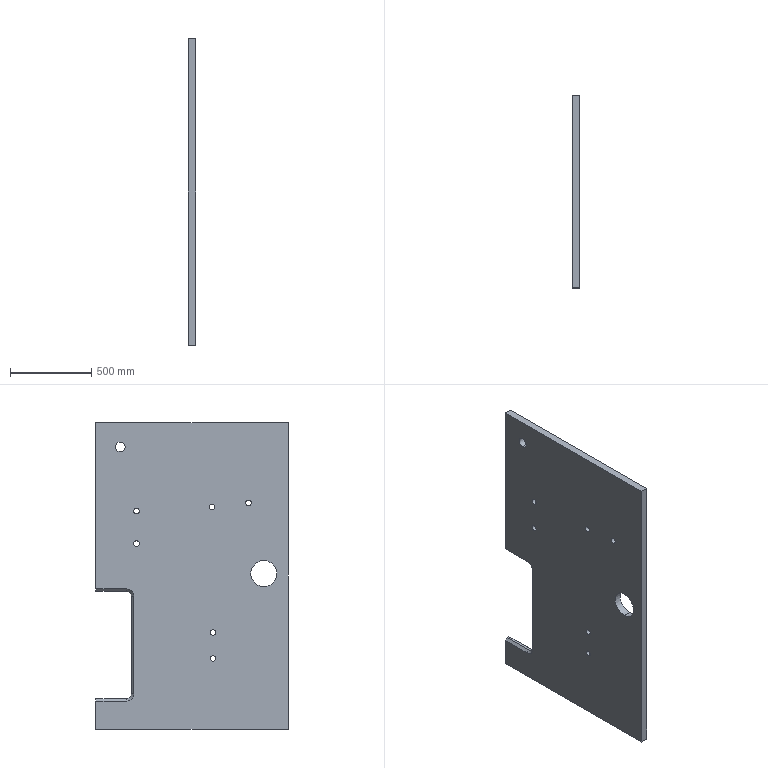Part | SolidWorks | features ICE 2, Chamfer 1, Extrusion 1, Fillet 1 | 1 solid | 38 faces | box 45 x 1185 x 1890 mm | volume 92721344 mm3 | cylinder 18 | plane 16 | cone 4 | commonest cylinder face diameters 35 x8 33 x4 60 x2 62 x2 160 x2
STEP:
#1=CARTESIAN_POINT('',(-22.5,463.,-66.5));
#2=VERTEX_POINT('',#1);
#3=CARTESIAN_POINT('',(-22.5,463.,-99.5));
#4=VERTEX_POINT('',#3);
#5=CARTESIAN_POINT('',(-22.5,463.,-83.));
#6=DIRECTION('',(1.,0.,0.));
#7=DIRECTION('',(0.,0.,-1.));
#8=AXIS2_PLACEMENT_3D('',#5,#6,#7);
#9=CIRCLE('',#8,16.5);
#10=EDGE_CURVE('',#2,#4,#9,.T.);
#11=ORIENTED_EDGE('',*,*,#10,.F.);
#12=CARTESIAN_POINT('',(22.5,463.,-66.5));
#13=VERTEX_POINT('',#12);
#14=CARTESIAN_POINT('',(-136.5,463.,-66.5));
#15=DIRECTION('',(1.,0.,0.));
#16=VECTOR('',#15,1000.);
#17=LINE('',#14,#16);
#18=EDGE_CURVE('',#2,#13,#17,.T.);
#19=ORIENTED_EDGE('',*,*,#18,.T.);
#20=CARTESIAN_POINT('',(22.5,463.,-99.5));
#21=VERTEX_POINT('',#20);
#22=CARTESIAN_POINT('',(22.5,463.,-83.));
#23=DIRECTION('',(1.,0.,0.));
#24=DIRECTION('',(0.,0.,-1.));
#25=AXIS2_PLACEMENT_3D('',#22,#23,#24);
#26=CIRCLE('',#25,16.5);
#27=EDGE_CURVE('',#13,#21,#26,.T.);
#28=ORIENTED_EDGE('',*,*,#27,.T.);
#29=CARTESIAN_POINT('',(-136.5,463.,-99.5));
#30=DIRECTION('',(1.,0.,0.));
#31=VECTOR('',#30,1000.);
#32=LINE('',#29,#31);
#33=EDGE_CURVE('',#4,#21,#32,.T.);
#34=ORIENTED_EDGE('',*,*,#33,.F.);
#35=EDGE_LOOP('',(#11,#19,#28,#34));
#36=FACE_OUTER_BOUND('',#35,.T.);
#37=CARTESIAN_POINT('',(-136.5,463.,-83.));
#38=DIRECTION('',(1.,0.,0.));
#39=DIRECTION('',(0.,0.,-1.));
#40=AXIS2_PLACEMENT_3D('',#37,#38,#39);
#41=CYLINDRICAL_SURFACE('',#40,16.5);
#42=ADVANCED_FACE('',(#36),#41,.F.);
#43=CARTESIAN_POINT('',(-22.5,463.,93.5));
#44=VERTEX_POINT('',#43);
#45=CARTESIAN_POINT('',(-22.5,463.,60.5));
#46=VERTEX_POINT('',#45);
#47=CARTESIAN_POINT('',(-22.5,463.,77.));
#48=DIRECTION('',(1.,0.,0.));
#49=DIRECTION('',(0.,0.,-1.));
#50=AXIS2_PLACEMENT_3D('',#47,#48,#49);
#51=CIRCLE('',#50,16.5);
#52=EDGE_CURVE('',#44,#46,#51,.T.);
#53=ORIENTED_EDGE('',*,*,#52,.F.);
#54=CARTESIAN_POINT('',(22.5,463.,93.5));
#55=VERTEX_POINT('',#54);
#56=CARTESIAN_POINT('',(-136.5,463.,93.5));
#57=DIRECTION('',(1.,0.,0.));
#58=VECTOR('',#57,1000.);
#59=LINE('',#56,#58);
#60=EDGE_CURVE('',#44,#55,#59,.T.);
#61=ORIENTED_EDGE('',*,*,#60,.T.);
#62=CARTESIAN_POINT('',(22.5,463.,60.5));
#63=VERTEX_POINT('',#62);
#64=CARTESIAN_POINT('',(22.5,463.,77.));
#65=DIRECTION('',(1.,0.,0.));
#66=DIRECTION('',(0.,0.,-1.));
#67=AXIS2_PLACEMENT_3D('',#64,#65,#66);
#68=CIRCLE('',#67,16.5);
#69=EDGE_CURVE('',#55,#63,#68,.T.);
#70=ORIENTED_EDGE('',*,*,#69,.T.);
#71=CARTESIAN_POINT('',(-136.5,463.,60.5));
#72=DIRECTION('',(1.,0.,0.));
#73=VECTOR('',#72,1000.);
#74=LINE('',#71,#73);
#75=EDGE_CURVE('',#46,#63,#74,.T.);
#76=ORIENTED_EDGE('',*,*,#75,.F.);
#77=EDGE_LOOP('',(#53,#61,#70,#76));
#78=FACE_OUTER_BOUND('',#77,.T.);
#79=CARTESIAN_POINT('',(-136.5,463.,77.));
#80=DIRECTION('',(1.,0.,0.));
#81=DIRECTION('',(0.,0.,-1.));
#82=AXIS2_PLACEMENT_3D('',#79,#80,#81);
#83=CYLINDRICAL_SURFACE('',#82,16.5);
#84=ADVANCED_FACE('',(#78),#83,.F.);
#85=CARTESIAN_POINT('',(-22.5,935.,842.5));
#86=VERTEX_POINT('',#85);
#87=CARTESIAN_POINT('',(-22.5,935.,807.5));
#88=VERTEX_POINT('',#87);
#89=CARTESIAN_POINT('',(-22.5,935.,825.));
#90=DIRECTION('',(1.,0.,0.));
#91=DIRECTION('',(0.,0.,-1.));
#92=AXIS2_PLACEMENT_3D('',#89,#90,#91);
#93=CIRCLE('',#92,17.5);
#94=EDGE_CURVE('',#86,#88,#93,.T.);
#95=ORIENTED_EDGE('',*,*,#94,.F.);
#96=CARTESIAN_POINT('',(22.5,935.,842.5));
#97=VERTEX_POINT('',#96);
#98=CARTESIAN_POINT('',(-22.5,935.,842.5));
#99=DIRECTION('',(1.,0.,0.));
#100=VECTOR('',#99,1000.);
#101=LINE('',#98,#100);
#102=EDGE_CURVE('',#86,#97,#101,.T.);
#103=ORIENTED_EDGE('',*,*,#102,.T.);
#104=CARTESIAN_POINT('',(22.5,935.,807.5));
#105=VERTEX_POINT('',#104);
#106=CARTESIAN_POINT('',(22.5,935.,825.));
#107=DIRECTION('',(1.,0.,0.));
#108=DIRECTION('',(0.,0.,-1.));
#109=AXIS2_PLACEMENT_3D('',#106,#107,#108);
#110=CIRCLE('',#109,17.5);
#111=EDGE_CURVE('',#97,#105,#110,.T.);
#112=ORIENTED_EDGE('',*,*,#111,.T.);
#113=CARTESIAN_POINT('',(-22.5,935.,807.5));
#114=DIRECTION('',(1.,0.,0.));
#115=VECTOR('',#114,1000.);
#116=LINE('',#113,#115);
#117=EDGE_CURVE('',#88,#105,#116,.T.);
#118=ORIENTED_EDGE('',*,*,#117,.F.);
#119=EDGE_LOOP('',(#95,#103,#112,#118));
#120=FACE_OUTER_BOUND('',#119,.T.);
#121=CARTESIAN_POINT('',(-22.5,935.,825.));
#122=DIRECTION('',(1.,0.,0.));
#123=DIRECTION('',(0.,0.,-1.));
#124=AXIS2_PLACEMENT_3D('',#121,#122,#123);
#125=CYLINDRICAL_SURFACE('',#124,17.5);
#126=ADVANCED_FACE('',(#120),#125,.F.);
#127=CARTESIAN_POINT('',(-22.5,935.,642.5));
#128=VERTEX_POINT('',#127);
#129=CARTESIAN_POINT('',(-22.5,935.,607.5));
#130=VERTEX_POINT('',#129);
#131=CARTESIAN_POINT('',(-22.5,935.,625.));
#132=DIRECTION('',(1.,0.,0.));
#133=DIRECTION('',(0.,0.,-1.));
#134=AXIS2_PLACEMENT_3D('',#131,#132,#133);
#135=CIRCLE('',#134,17.5);
#136=EDGE_CURVE('',#128,#130,#135,.T.);
#137=ORIENTED_EDGE('',*,*,#136,.F.);
#138=CARTESIAN_POINT('',(22.5,935.,642.5));
#139=VERTEX_POINT('',#138);
#140=CARTESIAN_POINT('',(-22.5,935.,642.5));
#141=DIRECTION('',(1.,0.,0.));
#142=VECTOR('',#141,1000.);
#143=LINE('',#140,#142);
#144=EDGE_CURVE('',#128,#139,#143,.T.);
#145=ORIENTED_EDGE('',*,*,#144,.T.);
#146=CARTESIAN_POINT('',(22.5,935.,607.5));
#147=VERTEX_POINT('',#146);
#148=CARTESIAN_POINT('',(22.5,935.,625.));
#149=DIRECTION('',(1.,0.,0.));
#150=DIRECTION('',(0.,0.,-1.));
#151=AXIS2_PLACEMENT_3D('',#148,#149,#150);
#152=CIRCLE('',#151,17.5);
#153=EDGE_CURVE('',#139,#147,#152,.T.);
#154=ORIENTED_EDGE('',*,*,#153,.T.);
#155=CARTESIAN_POINT('',(-22.5,935.,607.5));
#156=DIRECTION('',(1.,0.,0.));
#157=VECTOR('',#156,1000.);
#158=LINE('',#155,#157);
#159=EDGE_CURVE('',#130,#147,#158,.T.);
#160=ORIENTED_EDGE('',*,*,#159,.F.);
#161=EDGE_LOOP('',(#137,#145,#154,#160));
#162=FACE_OUTER_BOUND('',#161,.T.);
#163=CARTESIAN_POINT('',(-22.5,935.,625.));
#164=DIRECTION('',(1.,0.,0.));
#165=DIRECTION('',(0.,0.,-1.));
#166=AXIS2_PLACEMENT_3D('',#163,#164,#165);
#167=CYLINDRICAL_SURFACE('',#166,17.5);
#168=ADVANCED_FACE('',(#162),#167,.F.);
#169=CARTESIAN_POINT('',(-22.5,470.,867.5));
#170=VERTEX_POINT('',#169);
#171=CARTESIAN_POINT('',(-22.5,470.,832.5));
#172=VERTEX_POINT('',#171);
#173=CARTESIAN_POINT('',(-22.5,470.,850.));
#174=DIRECTION('',(1.,0.,0.));
#175=DIRECTION('',(0.,0.,-1.));
#176=AXIS2_PLACEMENT_3D('',#173,#174,#175);
#177=CIRCLE('',#176,17.5);
#178=EDGE_CURVE('',#170,#172,#177,.T.);
#179=ORIENTED_EDGE('',*,*,#178,.F.);
#180=CARTESIAN_POINT('',(22.5,470.,867.5));
#181=VERTEX_POINT('',#180);
#182=CARTESIAN_POINT('',(-22.5,470.,867.5));
#183=DIRECTION('',(1.,0.,0.));
#184=VECTOR('',#183,1000.);
#185=LINE('',#182,#184);
#186=EDGE_CURVE('',#170,#181,#185,.T.);
#187=ORIENTED_EDGE('',*,*,#186,.T.);
#188=CARTESIAN_POINT('',(22.5,470.,832.5));
#189=VERTEX_POINT('',#188);
#190=CARTESIAN_POINT('',(22.5,470.,850.));
#191=DIRECTION('',(1.,0.,0.));
#192=DIRECTION('',(0.,0.,-1.));
#193=AXIS2_PLACEMENT_3D('',#190,#191,#192);
#194=CIRCLE('',#193,17.5);
#195=EDGE_CURVE('',#181,#189,#194,.T.);
#196=ORIENTED_EDGE('',*,*,#195,.T.);
#197=CARTESIAN_POINT('',(-22.5,470.,832.5));
#198=DIRECTION('',(1.,0.,0.));
#199=VECTOR('',#198,1000.);
#200=LINE('',#197,#199);
#201=EDGE_CURVE('',#172,#189,#200,.T.);
#202=ORIENTED_EDGE('',*,*,#201,.F.);
#203=EDGE_LOOP('',(#179,#187,#196,#202));
#204=FACE_OUTER_BOUND('',#203,.T.);
#205=CARTESIAN_POINT('',(-22.5,470.,850.));
#206=DIRECTION('',(1.,0.,0.));
#207=DIRECTION('',(0.,0.,-1.));
#208=AXIS2_PLACEMENT_3D('',#205,#206,#207);
#209=CYLINDRICAL_SURFACE('',#208,17.5);
#210=ADVANCED_FACE('',(#204),#209,.F.);
#211=CARTESIAN_POINT('',(-22.5,245.,892.5));
#212=VERTEX_POINT('',#211);
#213=CARTESIAN_POINT('',(-22.5,245.,857.5));
#214=VERTEX_POINT('',#213);
#215=CARTESIAN_POINT('',(-22.5,245.,875.));
#216=DIRECTION('',(1.,0.,0.));
#217=DIRECTION('',(0.,0.,-1.));
#218=AXIS2_PLACEMENT_3D('',#215,#216,#217);
#219=CIRCLE('',#218,17.5);
#220=EDGE_CURVE('',#212,#214,#219,.T.);
#221=ORIENTED_EDGE('',*,*,#220,.F.);
#222=CARTESIAN_POINT('',(22.5,245.,892.5));
#223=VERTEX_POINT('',#222);
#224=CARTESIAN_POINT('',(-22.5,245.,892.5));
#225=DIRECTION('',(1.,0.,0.));
#226=VECTOR('',#225,1000.);
#227=LINE('',#224,#226);
#228=EDGE_CURVE('',#212,#223,#227,.T.);
#229=ORIENTED_EDGE('',*,*,#228,.T.);
#230=CARTESIAN_POINT('',(22.5,245.,857.5));
#231=VERTEX_POINT('',#230);
#232=CARTESIAN_POINT('',(22.5,245.,875.));
#233=DIRECTION('',(1.,0.,0.));
#234=DIRECTION('',(0.,0.,-1.));
#235=AXIS2_PLACEMENT_3D('',#232,#233,#234);
#236=CIRCLE('',#235,17.5);
#237=EDGE_CURVE('',#223,#231,#236,.T.);
#238=ORIENTED_EDGE('',*,*,#237,.T.);
#239=CARTESIAN_POINT('',(-22.5,245.,857.5));
#240=DIRECTION('',(1.,0.,0.));
#241=VECTOR('',#240,1000.);
#242=LINE('',#239,#241);
#243=EDGE_CURVE('',#214,#231,#242,.T.);
#244=ORIENTED_EDGE('',*,*,#243,.F.);
#245=EDGE_LOOP('',(#221,#229,#238,#244));
#246=FACE_OUTER_BOUND('',#245,.T.);
#247=CARTESIAN_POINT('',(-22.5,245.,875.));
#248=DIRECTION('',(1.,0.,0.));
#249=DIRECTION('',(0.,0.,-1.));
#250=AXIS2_PLACEMENT_3D('',#247,#248,#249);
#251=CYLINDRICAL_SURFACE('',#250,17.5);
#252=ADVANCED_FACE('',(#246),#251,.F.);
#253=CARTESIAN_POINT('',(-22.5,150.,520.));
#254=VERTEX_POINT('',#253);
#255=CARTESIAN_POINT('',(-22.5,150.,360.));
#256=VERTEX_POINT('',#255);
#257=CARTESIAN_POINT('',(-22.5,150.,440.));
#258=DIRECTION('',(1.,0.,0.));
#259=DIRECTION('',(0.,0.,-1.));
#260=AXIS2_PLACEMENT_3D('',#257,#258,#259);
#261=CIRCLE('',#260,80.);
#262=EDGE_CURVE('',#254,#256,#261,.T.);
#263=ORIENTED_EDGE('',*,*,#262,.F.);
#264=CARTESIAN_POINT('',(22.5,150.,520.));
#265=VERTEX_POINT('',#264);
#266=CARTESIAN_POINT('',(-22.5,150.,520.));
#267=DIRECTION('',(1.,0.,0.));
#268=VECTOR('',#267,1000.);
#269=LINE('',#266,#268);
#270=EDGE_CURVE('',#254,#265,#269,.T.);
#271=ORIENTED_EDGE('',*,*,#270,.T.);
#272=CARTESIAN_POINT('',(22.5,150.,360.));
#273=VERTEX_POINT('',#272);
#274=CARTESIAN_POINT('',(22.5,150.,440.));
#275=DIRECTION('',(1.,0.,0.));
#276=DIRECTION('',(0.,0.,-1.));
#277=AXIS2_PLACEMENT_3D('',#274,#275,#276);
#278=CIRCLE('',#277,80.);
#279=EDGE_CURVE('',#265,#273,#278,.T.);
#280=ORIENTED_EDGE('',*,*,#279,.T.);
#281=CARTESIAN_POINT('',(-22.5,150.,360.));
#282=DIRECTION('',(1.,0.,0.));
#283=VECTOR('',#282,1000.);
#284=LINE('',#281,#283);
#285=EDGE_CURVE('',#256,#273,#284,.T.);
#286=ORIENTED_EDGE('',*,*,#285,.F.);
#287=EDGE_LOOP('',(#263,#271,#280,#286));
#288=FACE_OUTER_BOUND('',#287,.T.);
#289=CARTESIAN_POINT('',(-22.5,150.,440.));
#290=DIRECTION('',(1.,0.,0.));
#291=DIRECTION('',(0.,0.,-1.));
#292=AXIS2_PLACEMENT_3D('',#289,#290,#291);
#293=CYLINDRICAL_SURFACE('',#292,80.);
#294=ADVANCED_FACE('',(#288),#293,.F.);
#295=CARTESIAN_POINT('',(-22.5,1035.,1250.));
#296=VERTEX_POINT('',#295);
#297=CARTESIAN_POINT('',(-22.5,1035.,1190.));
#298=VERTEX_POINT('',#297);
#299=CARTESIAN_POINT('',(-22.5,1035.,1220.));
#300=DIRECTION('',(1.,0.,0.));
#301=DIRECTION('',(0.,0.,-1.));
#302=AXIS2_PLACEMENT_3D('',#299,#300,#301);
#303=CIRCLE('',#302,30.);
#304=EDGE_CURVE('',#296,#298,#303,.T.);
#305=ORIENTED_EDGE('',*,*,#304,.F.);
#306=CARTESIAN_POINT('',(22.5,1035.,1250.));
#307=VERTEX_POINT('',#306);
#308=CARTESIAN_POINT('',(-22.5,1035.,1250.));
#309=DIRECTION('',(1.,0.,0.));
#310=VECTOR('',#309,1000.);
#311=LINE('',#308,#310);
#312=EDGE_CURVE('',#296,#307,#311,.T.);
#313=ORIENTED_EDGE('',*,*,#312,.T.);
#314=CARTESIAN_POINT('',(22.5,1035.,1190.));
#315=VERTEX_POINT('',#314);
#316=CARTESIAN_POINT('',(22.5,1035.,1220.));
#317=DIRECTION('',(1.,0.,0.));
#318=DIRECTION('',(0.,0.,-1.));
#319=AXIS2_PLACEMENT_3D('',#316,#317,#318);
#320=CIRCLE('',#319,30.);
#321=EDGE_CURVE('',#307,#315,#320,.T.);
#322=ORIENTED_EDGE('',*,*,#321,.T.);
#323=CARTESIAN_POINT('',(-22.5,1035.,1190.));
#324=DIRECTION('',(1.,0.,0.));
#325=VECTOR('',#324,1000.);
#326=LINE('',#323,#325);
#327=EDGE_CURVE('',#298,#315,#326,.T.);
#328=ORIENTED_EDGE('',*,*,#327,.F.);
#329=EDGE_LOOP('',(#305,#313,#322,#328));
#330=FACE_OUTER_BOUND('',#329,.T.);
#331=CARTESIAN_POINT('',(-22.5,1035.,1220.));
#332=DIRECTION('',(1.,0.,0.));
#333=DIRECTION('',(0.,0.,-1.));
#334=AXIS2_PLACEMENT_3D('',#331,#332,#333);
#335=CYLINDRICAL_SURFACE('',#334,30.);
#336=ADVANCED_FACE('',(#330),#335,.F.);
#337=CARTESIAN_POINT('',(-22.5,0.,1370.));
#338=VERTEX_POINT('',#337);
#339=CARTESIAN_POINT('',(-22.5,0.,-520.));
#340=VERTEX_POINT('',#339);
#341=CARTESIAN_POINT('',(-22.5,0.,0.));
#342=DIRECTION('',(0.,0.,-1.));
#343=VECTOR('',#342,1000.);
#344=LINE('',#341,#343);
#345=EDGE_CURVE('',#338,#340,#344,.T.);
#346=ORIENTED_EDGE('',*,*,#345,.T.);
#347=CARTESIAN_POINT('',(22.5,0.,-520.));
#348=VERTEX_POINT('',#347);
#349=CARTESIAN_POINT('',(22.5,0.,-520.));
#350=DIRECTION('',(-1.,0.,0.));
#351=VECTOR('',#350,1000.);
#352=LINE('',#349,#351);
#353=EDGE_CURVE('',#348,#340,#352,.T.);
#354=ORIENTED_EDGE('',*,*,#353,.F.);
#355=CARTESIAN_POINT('',(22.5,0.,1370.));
#356=VERTEX_POINT('',#355);
#357=CARTESIAN_POINT('',(22.5,0.,1370.));
#358=DIRECTION('',(0.,0.,-1.));
#359=VECTOR('',#358,1000.);
#360=LINE('',#357,#359);
#361=EDGE_CURVE('',#356,#348,#360,.T.);
#362=ORIENTED_EDGE('',*,*,#361,.F.);
#363=CARTESIAN_POINT('',(22.5,0.,1370.));
#364=DIRECTION('',(-1.,0.,0.));
#365=VECTOR('',#364,1000.);
#366=LINE('',#363,#365);
#367=EDGE_CURVE('',#356,#338,#366,.T.);
#368=ORIENTED_EDGE('',*,*,#367,.T.);
#369=EDGE_LOOP('',(#346,#354,#362,#368));
#370=FACE_OUTER_BOUND('',#369,.T.);
#371=CARTESIAN_POINT('',(22.5,0.,0.));
#372=DIRECTION('',(0.,1.,0.));
#373=DIRECTION('',(0.,0.,1.));
#374=AXIS2_PLACEMENT_3D('',#371,#372,#373);
#375=PLANE('',#374);
#376=ADVANCED_FACE('',(#370),#375,.F.);
#377=CARTESIAN_POINT('',(-22.5,1185.,-520.));
#378=VERTEX_POINT('',#377);
#379=CARTESIAN_POINT('',(-22.5,0.,-520.));
#380=DIRECTION('',(0.,1.,0.));
#381=VECTOR('',#380,1000.);
#382=LINE('',#379,#381);
#383=EDGE_CURVE('',#340,#378,#382,.T.);
#384=ORIENTED_EDGE('',*,*,#383,.T.);
#385=CARTESIAN_POINT('',(22.5,1185.,-520.));
#386=VERTEX_POINT('',#385);
#387=CARTESIAN_POINT('',(22.5,1185.,-520.));
#388=DIRECTION('',(-1.,0.,0.));
#389=VECTOR('',#388,1000.);
#390=LINE('',#387,#389);
#391=EDGE_CURVE('',#386,#378,#390,.T.);
#392=ORIENTED_EDGE('',*,*,#391,.F.);
#393=CARTESIAN_POINT('',(22.5,0.,-520.));
#394=DIRECTION('',(0.,1.,0.));
#395=VECTOR('',#394,1000.);
#396=LINE('',#393,#395);
#397=EDGE_CURVE('',#348,#386,#396,.T.);
#398=ORIENTED_EDGE('',*,*,#397,.F.);
#399=ORIENTED_EDGE('',*,*,#353,.T.);
#400=EDGE_LOOP('',(#384,#392,#398,#399));
#401=FACE_OUTER_BOUND('',#400,.T.);
#402=CARTESIAN_POINT('',(22.5,0.,-520.));
#403=DIRECTION('',(0.,0.,1.));
#404=DIRECTION('',(1.,0.,0.));
#405=AXIS2_PLACEMENT_3D('',#402,#403,#404);
#406=PLANE('',#405);
#407=ADVANCED_FACE('',(#401),#406,.F.);
#408=CARTESIAN_POINT('',(-22.5,1185.,-346.));
#409=VERTEX_POINT('',#408);
#410=CARTESIAN_POINT('',(-22.5,1185.,-520.));
#411=DIRECTION('',(0.,0.,1.));
#412=VECTOR('',#411,1000.);
#413=LINE('',#410,#412);
#414=EDGE_CURVE('',#378,#409,#413,.T.);
#415=ORIENTED_EDGE('',*,*,#414,.T.);
#416=CARTESIAN_POINT('',(-7.5,1185.,-331.));
#417=VERTEX_POINT('',#416);
#418=CARTESIAN_POINT('',(-7.5,1185.,-331.));
#419=DIRECTION('',(0.7071,0.,0.7071));
#420=VECTOR('',#419,1000.);
#421=LINE('',#418,#420);
#422=EDGE_CURVE('',#409,#417,#421,.T.);
#423=ORIENTED_EDGE('',*,*,#422,.T.);
#424=CARTESIAN_POINT('',(7.5,1185.,-331.));
#425=VERTEX_POINT('',#424);
#426=CARTESIAN_POINT('',(22.5,1185.,-331.));
#427=DIRECTION('',(-1.,0.,0.));
#428=VECTOR('',#427,1000.);
#429=LINE('',#426,#428);
#430=EDGE_CURVE('',#425,#417,#429,.T.);
#431=ORIENTED_EDGE('',*,*,#430,.F.);
#432=CARTESIAN_POINT('',(22.5,1185.,-346.));
#433=VERTEX_POINT('',#432);
#434=CARTESIAN_POINT('',(22.5,1185.,-346.));
#435=DIRECTION('',(0.7071,0.,-0.7071));
#436=VECTOR('',#435,1000.);
#437=LINE('',#434,#436);
#438=EDGE_CURVE('',#425,#433,#437,.T.);
#439=ORIENTED_EDGE('',*,*,#438,.T.);
#440=CARTESIAN_POINT('',(22.5,1185.,-520.));
#441=DIRECTION('',(0.,0.,1.));
#442=VECTOR('',#441,1000.);
#443=LINE('',#440,#442);
#444=EDGE_CURVE('',#386,#433,#443,.T.);
#445=ORIENTED_EDGE('',*,*,#444,.F.);
#446=ORIENTED_EDGE('',*,*,#391,.T.);
#447=EDGE_LOOP('',(#415,#423,#431,#439,#445,#446));
#448=FACE_OUTER_BOUND('',#447,.T.);
#449=CARTESIAN_POINT('',(22.5,1185.,-520.));
#450=DIRECTION('',(0.,-1.,0.));
#451=DIRECTION('',(0.,0.,-1.));
#452=AXIS2_PLACEMENT_3D('',#449,#450,#451);
#453=PLANE('',#452);
#454=ADVANCED_FACE('',(#448),#453,.F.);
#455=ORIENTED_EDGE('',*,*,#430,.T.);
#456=CARTESIAN_POINT('',(-7.5,996.,-331.));
#457=VERTEX_POINT('',#456);
#458=CARTESIAN_POINT('',(-7.5,1185.,-331.));
#459=DIRECTION('',(0.,-1.,0.));
#460=VECTOR('',#459,1000.);
#461=LINE('',#458,#460);
#462=EDGE_CURVE('',#417,#457,#461,.T.);
#463=ORIENTED_EDGE('',*,*,#462,.T.);
#464=CARTESIAN_POINT('',(7.5,996.,-331.));
#465=VERTEX_POINT('',#464);
#466=CARTESIAN_POINT('',(22.5,996.,-331.));
#467=DIRECTION('',(1.,0.,0.));
#468=VECTOR('',#467,1000.);
#469=LINE('',#466,#468);
#470=EDGE_CURVE('',#457,#465,#469,.T.);
#471=ORIENTED_EDGE('',*,*,#470,.T.);
#472=CARTESIAN_POINT('',(7.5,1185.,-331.));
#473=DIRECTION('',(0.,1.,0.));
#474=VECTOR('',#473,1000.);
#475=LINE('',#472,#474);
#476=EDGE_CURVE('',#465,#425,#475,.T.);
#477=ORIENTED_EDGE('',*,*,#476,.T.);
#478=EDGE_LOOP('',(#455,#463,#471,#477));
#479=FACE_OUTER_BOUND('',#478,.T.);
#480=CARTESIAN_POINT('',(22.5,1185.,-331.));
#481=DIRECTION('',(0.,0.,-1.));
#482=DIRECTION('',(-1.,0.,0.));
#483=AXIS2_PLACEMENT_3D('',#480,#481,#482);
#484=PLANE('',#483);
#485=ADVANCED_FACE('',(#479),#484,.F.);
#486=CARTESIAN_POINT('',(7.5,965.,-300.));
#487=VERTEX_POINT('',#486);
#488=CARTESIAN_POINT('',(-7.5,965.,-300.));
#489=VERTEX_POINT('',#488);
#490=CARTESIAN_POINT('',(-22.5,965.,-300.));
#491=DIRECTION('',(-1.,0.,0.));
#492=VECTOR('',#491,1000.);
#493=LINE('',#490,#492);
#494=EDGE_CURVE('',#487,#489,#493,.T.);
#495=ORIENTED_EDGE('',*,*,#494,.T.);
#496=CARTESIAN_POINT('',(-7.5,965.,300.));
#497=VERTEX_POINT('',#496);
#498=CARTESIAN_POINT('',(-7.5,965.,-331.));
#499=DIRECTION('',(0.,0.,1.));
#500=VECTOR('',#499,1000.);
#501=LINE('',#498,#500);
#502=EDGE_CURVE('',#489,#497,#501,.T.);
#503=ORIENTED_EDGE('',*,*,#502,.T.);
#504=CARTESIAN_POINT('',(7.5,965.,300.));
#505=VERTEX_POINT('',#504);
#506=CARTESIAN_POINT('',(22.5,965.,300.));
#507=DIRECTION('',(1.,0.,0.));
#508=VECTOR('',#507,1000.);
#509=LINE('',#506,#508);
#510=EDGE_CURVE('',#497,#505,#509,.T.);
#511=ORIENTED_EDGE('',*,*,#510,.T.);
#512=CARTESIAN_POINT('',(7.5,965.,-300.));
#513=DIRECTION('',(0.,0.,-1.));
#514=VECTOR('',#513,1000.);
#515=LINE('',#512,#514);
#516=EDGE_CURVE('',#505,#487,#515,.T.);
#517=ORIENTED_EDGE('',*,*,#516,.T.);
#518=EDGE_LOOP('',(#495,#503,#511,#517));
#519=FACE_OUTER_BOUND('',#518,.T.);
#520=CARTESIAN_POINT('',(22.5,965.,-331.));
#521=DIRECTION('',(0.,-1.,0.));
#522=DIRECTION('',(0.,0.,-1.));
#523=AXIS2_PLACEMENT_3D('',#520,#521,#522);
#524=PLANE('',#523);
#525=ADVANCED_FACE('',(#519),#524,.F.);
#526=CARTESIAN_POINT('',(7.5,996.,331.));
#527=VERTEX_POINT('',#526);
#528=CARTESIAN_POINT('',(-7.5,996.,331.));
#529=VERTEX_POINT('',#528);
#530=CARTESIAN_POINT('',(-22.5,996.,331.));
#531=DIRECTION('',(-1.,0.,0.));
#532=VECTOR('',#531,1000.);
#533=LINE('',#530,#532);
#534=EDGE_CURVE('',#527,#529,#533,.T.);
#535=ORIENTED_EDGE('',*,*,#534,.T.);
#536=CARTESIAN_POINT('',(-7.5,1185.,331.));
#537=VERTEX_POINT('',#536);
#538=CARTESIAN_POINT('',(-7.5,965.,331.));
#539=DIRECTION('',(0.,1.,0.));
#540=VECTOR('',#539,1000.);
#541=LINE('',#538,#540);
#542=EDGE_CURVE('',#529,#537,#541,.T.);
#543=ORIENTED_EDGE('',*,*,#542,.T.);
#544=CARTESIAN_POINT('',(7.5,1185.,331.));
#545=VERTEX_POINT('',#544);
#546=CARTESIAN_POINT('',(22.5,1185.,331.));
#547=DIRECTION('',(-1.,0.,0.));
#548=VECTOR('',#547,1000.);
#549=LINE('',#546,#548);
#550=EDGE_CURVE('',#545,#537,#549,.T.);
#551=ORIENTED_EDGE('',*,*,#550,.F.);
#552=CARTESIAN_POINT('',(7.5,996.,331.));
#553=DIRECTION('',(0.,-1.,0.));
#554=VECTOR('',#553,1000.);
#555=LINE('',#552,#554);
#556=EDGE_CURVE('',#545,#527,#555,.T.);
#557=ORIENTED_EDGE('',*,*,#556,.T.);
#558=EDGE_LOOP('',(#535,#543,#551,#557));
#559=FACE_OUTER_BOUND('',#558,.T.);
#560=CARTESIAN_POINT('',(22.5,965.,331.));
#561=DIRECTION('',(0.,0.,1.));
#562=DIRECTION('',(1.,0.,0.));
#563=AXIS2_PLACEMENT_3D('',#560,#561,#562);
#564=PLANE('',#563);
#565=ADVANCED_FACE('',(#559),#564,.F.);
#566=ORIENTED_EDGE('',*,*,#550,.T.);
#567=CARTESIAN_POINT('',(-22.5,1185.,346.));
#568=VERTEX_POINT('',#567);
#569=CARTESIAN_POINT('',(-7.5,1185.,331.));
#570=DIRECTION('',(-0.7071,0.,0.7071));
#571=VECTOR('',#570,1000.);
#572=LINE('',#569,#571);
#573=EDGE_CURVE('',#537,#568,#572,.T.);
#574=ORIENTED_EDGE('',*,*,#573,.T.);
#575=CARTESIAN_POINT('',(-22.5,1185.,1370.));
#576=VERTEX_POINT('',#575);
#577=CARTESIAN_POINT('',(-22.5,1185.,331.));
#578=DIRECTION('',(0.,0.,1.));
#579=VECTOR('',#578,1000.);
#580=LINE('',#577,#579);
#581=EDGE_CURVE('',#568,#576,#580,.T.);
#582=ORIENTED_EDGE('',*,*,#581,.T.);
#583=CARTESIAN_POINT('',(22.5,1185.,1370.));
#584=VERTEX_POINT('',#583);
#585=CARTESIAN_POINT('',(22.5,1185.,1370.));
#586=DIRECTION('',(-1.,0.,0.));
#587=VECTOR('',#586,1000.);
#588=LINE('',#585,#587);
#589=EDGE_CURVE('',#584,#576,#588,.T.);
#590=ORIENTED_EDGE('',*,*,#589,.F.);
#591=CARTESIAN_POINT('',(22.5,1185.,346.));
#592=VERTEX_POINT('',#591);
#593=CARTESIAN_POINT('',(22.5,1185.,331.));
#594=DIRECTION('',(0.,0.,1.));
#595=VECTOR('',#594,1000.);
#596=LINE('',#593,#595);
#597=EDGE_CURVE('',#592,#584,#596,.T.);
#598=ORIENTED_EDGE('',*,*,#597,.F.);
#599=CARTESIAN_POINT('',(22.5,1185.,346.));
#600=DIRECTION('',(-0.7071,0.,-0.7071));
#601=VECTOR('',#600,1000.);
#602=LINE('',#599,#601);
#603=EDGE_CURVE('',#592,#545,#602,.T.);
#604=ORIENTED_EDGE('',*,*,#603,.T.);
#605=EDGE_LOOP('',(#566,#574,#582,#590,#598,#604));
#606=FACE_OUTER_BOUND('',#605,.T.);
#607=CARTESIAN_POINT('',(22.5,1185.,331.));
#608=DIRECTION('',(0.,-1.,0.));
#609=DIRECTION('',(0.,0.,-1.));
#610=AXIS2_PLACEMENT_3D('',#607,#608,#609);
#611=PLANE('',#610);
#612=ADVANCED_FACE('',(#606),#611,.F.);
#613=CARTESIAN_POINT('',(-22.5,1185.,1370.));
#614=DIRECTION('',(0.,-1.,0.));
#615=VECTOR('',#614,1000.);
#616=LINE('',#613,#615);
#617=EDGE_CURVE('',#576,#338,#616,.T.);
#618=ORIENTED_EDGE('',*,*,#617,.T.);
#619=ORIENTED_EDGE('',*,*,#367,.F.);
#620=CARTESIAN_POINT('',(22.5,1185.,1370.));
#621=DIRECTION('',(0.,-1.,0.));
#622=VECTOR('',#621,1000.);
#623=LINE('',#620,#622);
#624=EDGE_CURVE('',#584,#356,#623,.T.);
#625=ORIENTED_EDGE('',*,*,#624,.F.);
#626=ORIENTED_EDGE('',*,*,#589,.T.);
#627=EDGE_LOOP('',(#618,#619,#625,#626));
#628=FACE_OUTER_BOUND('',#627,.T.);
#629=CARTESIAN_POINT('',(22.5,1185.,1370.));
#630=DIRECTION('',(0.,0.,-1.));
#631=DIRECTION('',(0.,1.,0.));
#632=AXIS2_PLACEMENT_3D('',#629,#630,#631);
#633=PLANE('',#632);
#634=ADVANCED_FACE('',(#628),#633,.F.);
#635=CARTESIAN_POINT('',(22.5,463.,-83.));
#636=DIRECTION('',(1.,0.,0.));
#637=DIRECTION('',(0.,0.,-1.));
#638=AXIS2_PLACEMENT_3D('',#635,#636,#637);
#639=CIRCLE('',#638,16.5);
#640=EDGE_CURVE('',#21,#13,#639,.T.);
#641=ORIENTED_EDGE('',*,*,#640,.F.);
#642=ORIENTED_EDGE('',*,*,#27,.F.);
#643=EDGE_LOOP('',(#641,#642));
#644=FACE_BOUND('',#643,.T.);
#645=CARTESIAN_POINT('',(22.5,463.,77.));
#646=DIRECTION('',(1.,0.,0.));
#647=DIRECTION('',(0.,0.,-1.));
#648=AXIS2_PLACEMENT_3D('',#645,#646,#647);
#649=CIRCLE('',#648,16.5);
#650=EDGE_CURVE('',#63,#55,#649,.T.);
#651=ORIENTED_EDGE('',*,*,#650,.F.);
#652=ORIENTED_EDGE('',*,*,#69,.F.);
#653=EDGE_LOOP('',(#651,#652));
#654=FACE_BOUND('',#653,.T.);
#655=CARTESIAN_POINT('',(22.5,935.,825.));
#656=DIRECTION('',(1.,0.,0.));
#657=DIRECTION('',(0.,0.,-1.));
#658=AXIS2_PLACEMENT_3D('',#655,#656,#657);
#659=CIRCLE('',#658,17.5);
#660=EDGE_CURVE('',#105,#97,#659,.T.);
#661=ORIENTED_EDGE('',*,*,#660,.F.);
#662=ORIENTED_EDGE('',*,*,#111,.F.);
#663=EDGE_LOOP('',(#661,#662));
#664=FACE_BOUND('',#663,.T.);
#665=CARTESIAN_POINT('',(22.5,935.,625.));
#666=DIRECTION('',(1.,0.,0.));
#667=DIRECTION('',(0.,0.,-1.));
#668=AXIS2_PLACEMENT_3D('',#665,#666,#667);
#669=CIRCLE('',#668,17.5);
#670=EDGE_CURVE('',#147,#139,#669,.T.);
#671=ORIENTED_EDGE('',*,*,#670,.F.);
#672=ORIENTED_EDGE('',*,*,#153,.F.);
#673=EDGE_LOOP('',(#671,#672));
#674=FACE_BOUND('',#673,.T.);
#675=CARTESIAN_POINT('',(22.5,470.,850.));
#676=DIRECTION('',(1.,0.,0.));
#677=DIRECTION('',(0.,0.,-1.));
#678=AXIS2_PLACEMENT_3D('',#675,#676,#677);
#679=CIRCLE('',#678,17.5);
#680=EDGE_CURVE('',#189,#181,#679,.T.);
#681=ORIENTED_EDGE('',*,*,#680,.F.);
#682=ORIENTED_EDGE('',*,*,#195,.F.);
#683=EDGE_LOOP('',(#681,#682));
#684=FACE_BOUND('',#683,.T.);
#685=CARTESIAN_POINT('',(22.5,245.,875.));
#686=DIRECTION('',(1.,0.,0.));
#687=DIRECTION('',(0.,0.,-1.));
#688=AXIS2_PLACEMENT_3D('',#685,#686,#687);
#689=CIRCLE('',#688,17.5);
#690=EDGE_CURVE('',#231,#223,#689,.T.);
#691=ORIENTED_EDGE('',*,*,#690,.F.);
#692=ORIENTED_EDGE('',*,*,#237,.F.);
#693=EDGE_LOOP('',(#691,#692));
#694=FACE_BOUND('',#693,.T.);
#695=CARTESIAN_POINT('',(22.5,150.,440.));
#696=DIRECTION('',(1.,0.,0.));
#697=DIRECTION('',(0.,0.,-1.));
#698=AXIS2_PLACEMENT_3D('',#695,#696,#697);
#699=CIRCLE('',#698,80.);
#700=EDGE_CURVE('',#273,#265,#699,.T.);
#701=ORIENTED_EDGE('',*,*,#700,.F.);
#702=ORIENTED_EDGE('',*,*,#279,.F.);
#703=EDGE_LOOP('',(#701,#702));
#704=FACE_BOUND('',#703,.T.);
#705=CARTESIAN_POINT('',(22.5,1035.,1220.));
#706=DIRECTION('',(1.,0.,0.));
#707=DIRECTION('',(0.,0.,-1.));
#708=AXIS2_PLACEMENT_3D('',#705,#706,#707);
#709=CIRCLE('',#708,30.);
#710=EDGE_CURVE('',#315,#307,#709,.T.);
#711=ORIENTED_EDGE('',*,*,#710,.F.);
#712=ORIENTED_EDGE('',*,*,#321,.F.);
#713=EDGE_LOOP('',(#711,#712));
#714=FACE_BOUND('',#713,.T.);
#715=ORIENTED_EDGE('',*,*,#444,.T.);
#716=CARTESIAN_POINT('',(22.5,996.,-346.));
#717=VERTEX_POINT('',#716);
#718=CARTESIAN_POINT('',(22.5,996.,-346.));
#719=DIRECTION('',(0.,-1.,0.));
#720=VECTOR('',#719,1000.);
#721=LINE('',#718,#720);
#722=EDGE_CURVE('',#433,#717,#721,.T.);
#723=ORIENTED_EDGE('',*,*,#722,.T.);
#724=CARTESIAN_POINT('',(22.5,950.,-300.));
#725=VERTEX_POINT('',#724);
#726=CARTESIAN_POINT('',(22.5,996.,-300.));
#727=DIRECTION('',(-1.,0.,0.));
#728=DIRECTION('',(0.,0.,-1.));
#729=AXIS2_PLACEMENT_3D('',#726,#727,#728);
#730=CIRCLE('',#729,46.);
#731=EDGE_CURVE('',#717,#725,#730,.T.);
#732=ORIENTED_EDGE('',*,*,#731,.T.);
#733=CARTESIAN_POINT('',(22.5,950.,300.));
#734=VERTEX_POINT('',#733);
#735=CARTESIAN_POINT('',(22.5,950.,300.));
#736=DIRECTION('',(0.,0.,1.));
#737=VECTOR('',#736,1000.);
#738=LINE('',#735,#737);
#739=EDGE_CURVE('',#725,#734,#738,.T.);
#740=ORIENTED_EDGE('',*,*,#739,.T.);
#741=CARTESIAN_POINT('',(22.5,996.,346.));
#742=VERTEX_POINT('',#741);
#743=CARTESIAN_POINT('',(22.5,996.,300.));
#744=DIRECTION('',(-1.,0.,0.));
#745=DIRECTION('',(0.,0.,-1.));
#746=AXIS2_PLACEMENT_3D('',#743,#744,#745);
#747=CIRCLE('',#746,46.);
#748=EDGE_CURVE('',#734,#742,#747,.T.);
#749=ORIENTED_EDGE('',*,*,#748,.T.);
#750=CARTESIAN_POINT('',(22.5,1185.,346.));
#751=DIRECTION('',(0.,1.,0.));
#752=VECTOR('',#751,1000.);
#753=LINE('',#750,#752);
#754=EDGE_CURVE('',#742,#592,#753,.T.);
#755=ORIENTED_EDGE('',*,*,#754,.T.);
#756=ORIENTED_EDGE('',*,*,#597,.T.);
#757=ORIENTED_EDGE('',*,*,#624,.T.);
#758=ORIENTED_EDGE('',*,*,#361,.T.);
#759=ORIENTED_EDGE('',*,*,#397,.T.);
#760=EDGE_LOOP('',(#715,#723,#732,#740,#749,#755,#756,#757,#758,#759));
#761=FACE_OUTER_BOUND('',#760,.T.);
#762=CARTESIAN_POINT('',(22.5,0.,0.));
#763=DIRECTION('',(1.,0.,0.));
#764=DIRECTION('',(0.,0.,-1.));
#765=AXIS2_PLACEMENT_3D('',#762,#763,#764);
#766=PLANE('',#765);
#767=ADVANCED_FACE('',(#644,#654,#664,#674,#684,#694,#704,#714,#761),#766,.T.);
#768=CARTESIAN_POINT('',(-22.5,463.,-83.));
#769=DIRECTION('',(1.,0.,0.));
#770=DIRECTION('',(0.,0.,-1.));
#771=AXIS2_PLACEMENT_3D('',#768,#769,#770);
#772=CIRCLE('',#771,16.5);
#773=EDGE_CURVE('',#4,#2,#772,.T.);
#774=ORIENTED_EDGE('',*,*,#773,.T.);
#775=ORIENTED_EDGE('',*,*,#10,.T.);
#776=EDGE_LOOP('',(#774,#775));
#777=FACE_BOUND('',#776,.T.);
#778=CARTESIAN_POINT('',(-22.5,463.,77.));
#779=DIRECTION('',(1.,0.,0.));
#780=DIRECTION('',(0.,0.,-1.));
#781=AXIS2_PLACEMENT_3D('',#778,#779,#780);
#782=CIRCLE('',#781,16.5);
#783=EDGE_CURVE('',#46,#44,#782,.T.);
#784=ORIENTED_EDGE('',*,*,#783,.T.);
#785=ORIENTED_EDGE('',*,*,#52,.T.);
#786=EDGE_LOOP('',(#784,#785));
#787=FACE_BOUND('',#786,.T.);
#788=CARTESIAN_POINT('',(-22.5,935.,825.));
#789=DIRECTION('',(1.,0.,0.));
#790=DIRECTION('',(0.,0.,-1.));
#791=AXIS2_PLACEMENT_3D('',#788,#789,#790);
#792=CIRCLE('',#791,17.5);
#793=EDGE_CURVE('',#88,#86,#792,.T.);
#794=ORIENTED_EDGE('',*,*,#793,.T.);
#795=ORIENTED_EDGE('',*,*,#94,.T.);
#796=EDGE_LOOP('',(#794,#795));
#797=FACE_BOUND('',#796,.T.);
#798=CARTESIAN_POINT('',(-22.5,935.,625.));
#799=DIRECTION('',(1.,0.,0.));
#800=DIRECTION('',(0.,0.,-1.));
#801=AXIS2_PLACEMENT_3D('',#798,#799,#800);
#802=CIRCLE('',#801,17.5);
#803=EDGE_CURVE('',#130,#128,#802,.T.);
#804=ORIENTED_EDGE('',*,*,#803,.T.);
#805=ORIENTED_EDGE('',*,*,#136,.T.);
#806=EDGE_LOOP('',(#804,#805));
#807=FACE_BOUND('',#806,.T.);
#808=CARTESIAN_POINT('',(-22.5,470.,850.));
#809=DIRECTION('',(1.,0.,0.));
#810=DIRECTION('',(0.,0.,-1.));
#811=AXIS2_PLACEMENT_3D('',#808,#809,#810);
#812=CIRCLE('',#811,17.5);
#813=EDGE_CURVE('',#172,#170,#812,.T.);
#814=ORIENTED_EDGE('',*,*,#813,.T.);
#815=ORIENTED_EDGE('',*,*,#178,.T.);
#816=EDGE_LOOP('',(#814,#815));
#817=FACE_BOUND('',#816,.T.);
#818=CARTESIAN_POINT('',(-22.5,245.,875.));
#819=DIRECTION('',(1.,0.,0.));
#820=DIRECTION('',(0.,0.,-1.));
#821=AXIS2_PLACEMENT_3D('',#818,#819,#820);
#822=CIRCLE('',#821,17.5);
#823=EDGE_CURVE('',#214,#212,#822,.T.);
#824=ORIENTED_EDGE('',*,*,#823,.T.);
#825=ORIENTED_EDGE('',*,*,#220,.T.);
#826=EDGE_LOOP('',(#824,#825));
#827=FACE_BOUND('',#826,.T.);
#828=CARTESIAN_POINT('',(-22.5,150.,440.));
#829=DIRECTION('',(1.,0.,0.));
#830=DIRECTION('',(0.,0.,-1.));
#831=AXIS2_PLACEMENT_3D('',#828,#829,#830);
#832=CIRCLE('',#831,80.);
#833=EDGE_CURVE('',#256,#254,#832,.T.);
#834=ORIENTED_EDGE('',*,*,#833,.T.);
#835=ORIENTED_EDGE('',*,*,#262,.T.);
#836=EDGE_LOOP('',(#834,#835));
#837=FACE_BOUND('',#836,.T.);
#838=CARTESIAN_POINT('',(-22.5,1035.,1220.));
#839=DIRECTION('',(1.,0.,0.));
#840=DIRECTION('',(0.,0.,-1.));
#841=AXIS2_PLACEMENT_3D('',#838,#839,#840);
#842=CIRCLE('',#841,30.);
#843=EDGE_CURVE('',#298,#296,#842,.T.);
#844=ORIENTED_EDGE('',*,*,#843,.T.);
#845=ORIENTED_EDGE('',*,*,#304,.T.);
#846=EDGE_LOOP('',(#844,#845));
#847=FACE_BOUND('',#846,.T.);
#848=ORIENTED_EDGE('',*,*,#581,.F.);
#849=CARTESIAN_POINT('',(-22.5,996.,346.));
#850=VERTEX_POINT('',#849);
#851=CARTESIAN_POINT('',(-22.5,0.,346.));
#852=DIRECTION('',(0.,-1.,0.));
#853=VECTOR('',#852,1000.);
#854=LINE('',#851,#853);
#855=EDGE_CURVE('',#568,#850,#854,.T.);
#856=ORIENTED_EDGE('',*,*,#855,.T.);
#857=CARTESIAN_POINT('',(-22.5,950.,300.));
#858=VERTEX_POINT('',#857);
#859=CARTESIAN_POINT('',(-22.5,996.,300.));
#860=DIRECTION('',(1.,0.,0.));
#861=DIRECTION('',(0.,0.,-1.));
#862=AXIS2_PLACEMENT_3D('',#859,#860,#861);
#863=CIRCLE('',#862,46.);
#864=EDGE_CURVE('',#850,#858,#863,.T.);
#865=ORIENTED_EDGE('',*,*,#864,.T.);
#866=CARTESIAN_POINT('',(-22.5,950.,-300.));
#867=VERTEX_POINT('',#866);
#868=CARTESIAN_POINT('',(-22.5,950.,0.));
#869=DIRECTION('',(0.,0.,-1.));
#870=VECTOR('',#869,1000.);
#871=LINE('',#868,#870);
#872=EDGE_CURVE('',#858,#867,#871,.T.);
#873=ORIENTED_EDGE('',*,*,#872,.T.);
#874=CARTESIAN_POINT('',(-22.5,996.,-346.));
#875=VERTEX_POINT('',#874);
#876=CARTESIAN_POINT('',(-22.5,996.,-300.));
#877=DIRECTION('',(1.,0.,0.));
#878=DIRECTION('',(0.,0.,-1.));
#879=AXIS2_PLACEMENT_3D('',#876,#877,#878);
#880=CIRCLE('',#879,46.);
#881=EDGE_CURVE('',#867,#875,#880,.T.);
#882=ORIENTED_EDGE('',*,*,#881,.T.);
#883=CARTESIAN_POINT('',(-22.5,0.,-346.));
#884=DIRECTION('',(0.,1.,0.));
#885=VECTOR('',#884,1000.);
#886=LINE('',#883,#885);
#887=EDGE_CURVE('',#875,#409,#886,.T.);
#888=ORIENTED_EDGE('',*,*,#887,.T.);
#889=ORIENTED_EDGE('',*,*,#414,.F.);
#890=ORIENTED_EDGE('',*,*,#383,.F.);
#891=ORIENTED_EDGE('',*,*,#345,.F.);
#892=ORIENTED_EDGE('',*,*,#617,.F.);
#893=EDGE_LOOP('',(#848,#856,#865,#873,#882,#888,#889,#890,#891,#892));
#894=FACE_OUTER_BOUND('',#893,.T.);
#895=CARTESIAN_POINT('',(-22.5,0.,0.));
#896=DIRECTION('',(1.,0.,0.));
#897=DIRECTION('',(0.,0.,-1.));
#898=AXIS2_PLACEMENT_3D('',#895,#896,#897);
#899=PLANE('',#898);
#900=ADVANCED_FACE('',(#777,#787,#797,#807,#817,#827,#837,#847,#894),#899,.F.);
#901=ORIENTED_EDGE('',*,*,#312,.F.);
#902=ORIENTED_EDGE('',*,*,#843,.F.);
#903=ORIENTED_EDGE('',*,*,#327,.T.);
#904=ORIENTED_EDGE('',*,*,#710,.T.);
#905=EDGE_LOOP('',(#901,#902,#903,#904));
#906=FACE_OUTER_BOUND('',#905,.T.);
#907=CARTESIAN_POINT('',(-22.5,1035.,1220.));
#908=DIRECTION('',(1.,0.,0.));
#909=DIRECTION('',(0.,0.,-1.));
#910=AXIS2_PLACEMENT_3D('',#907,#908,#909);
#911=CYLINDRICAL_SURFACE('',#910,30.);
#912=ADVANCED_FACE('',(#906),#911,.F.);
#913=ORIENTED_EDGE('',*,*,#270,.F.);
#914=ORIENTED_EDGE('',*,*,#833,.F.);
#915=ORIENTED_EDGE('',*,*,#285,.T.);
#916=ORIENTED_EDGE('',*,*,#700,.T.);
#917=EDGE_LOOP('',(#913,#914,#915,#916));
#918=FACE_OUTER_BOUND('',#917,.T.);
#919=CARTESIAN_POINT('',(-22.5,150.,440.));
#920=DIRECTION('',(1.,0.,0.));
#921=DIRECTION('',(0.,0.,-1.));
#922=AXIS2_PLACEMENT_3D('',#919,#920,#921);
#923=CYLINDRICAL_SURFACE('',#922,80.);
#924=ADVANCED_FACE('',(#918),#923,.F.);
#925=ORIENTED_EDGE('',*,*,#228,.F.);
#926=ORIENTED_EDGE('',*,*,#823,.F.);
#927=ORIENTED_EDGE('',*,*,#243,.T.);
#928=ORIENTED_EDGE('',*,*,#690,.T.);
#929=EDGE_LOOP('',(#925,#926,#927,#928));
#930=FACE_OUTER_BOUND('',#929,.T.);
#931=CARTESIAN_POINT('',(-22.5,245.,875.));
#932=DIRECTION('',(1.,0.,0.));
#933=DIRECTION('',(0.,0.,-1.));
#934=AXIS2_PLACEMENT_3D('',#931,#932,#933);
#935=CYLINDRICAL_SURFACE('',#934,17.5);
#936=ADVANCED_FACE('',(#930),#935,.F.);
#937=ORIENTED_EDGE('',*,*,#186,.F.);
#938=ORIENTED_EDGE('',*,*,#813,.F.);
#939=ORIENTED_EDGE('',*,*,#201,.T.);
#940=ORIENTED_EDGE('',*,*,#680,.T.);
#941=EDGE_LOOP('',(#937,#938,#939,#940));
#942=FACE_OUTER_BOUND('',#941,.T.);
#943=CARTESIAN_POINT('',(-22.5,470.,850.));
#944=DIRECTION('',(1.,0.,0.));
#945=DIRECTION('',(0.,0.,-1.));
#946=AXIS2_PLACEMENT_3D('',#943,#944,#945);
#947=CYLINDRICAL_SURFACE('',#946,17.5);
#948=ADVANCED_FACE('',(#942),#947,.F.);
#949=ORIENTED_EDGE('',*,*,#144,.F.);
#950=ORIENTED_EDGE('',*,*,#803,.F.);
#951=ORIENTED_EDGE('',*,*,#159,.T.);
#952=ORIENTED_EDGE('',*,*,#670,.T.);
#953=EDGE_LOOP('',(#949,#950,#951,#952));
#954=FACE_OUTER_BOUND('',#953,.T.);
#955=CARTESIAN_POINT('',(-22.5,935.,625.));
#956=DIRECTION('',(1.,0.,0.));
#957=DIRECTION('',(0.,0.,-1.));
#958=AXIS2_PLACEMENT_3D('',#955,#956,#957);
#959=CYLINDRICAL_SURFACE('',#958,17.5);
#960=ADVANCED_FACE('',(#954),#959,.F.);
#961=ORIENTED_EDGE('',*,*,#102,.F.);
#962=ORIENTED_EDGE('',*,*,#793,.F.);
#963=ORIENTED_EDGE('',*,*,#117,.T.);
#964=ORIENTED_EDGE('',*,*,#660,.T.);
#965=EDGE_LOOP('',(#961,#962,#963,#964));
#966=FACE_OUTER_BOUND('',#965,.T.);
#967=CARTESIAN_POINT('',(-22.5,935.,825.));
#968=DIRECTION('',(1.,0.,0.));
#969=DIRECTION('',(0.,0.,-1.));
#970=AXIS2_PLACEMENT_3D('',#967,#968,#969);
#971=CYLINDRICAL_SURFACE('',#970,17.5);
#972=ADVANCED_FACE('',(#966),#971,.F.);
#973=ORIENTED_EDGE('',*,*,#470,.F.);
#974=CARTESIAN_POINT('',(-7.5,996.,-300.));
#975=DIRECTION('',(-1.,0.,0.));
#976=DIRECTION('',(0.,0.,-1.));
#977=AXIS2_PLACEMENT_3D('',#974,#975,#976);
#978=CIRCLE('',#977,31.);
#979=EDGE_CURVE('',#457,#489,#978,.T.);
#980=ORIENTED_EDGE('',*,*,#979,.T.);
#981=ORIENTED_EDGE('',*,*,#494,.F.);
#982=CARTESIAN_POINT('',(7.5,996.,-300.));
#983=DIRECTION('',(1.,0.,0.));
#984=DIRECTION('',(0.,0.,-1.));
#985=AXIS2_PLACEMENT_3D('',#982,#983,#984);
#986=CIRCLE('',#985,31.);
#987=EDGE_CURVE('',#487,#465,#986,.T.);
#988=ORIENTED_EDGE('',*,*,#987,.T.);
#989=EDGE_LOOP('',(#973,#980,#981,#988));
#990=FACE_OUTER_BOUND('',#989,.T.);
#991=CARTESIAN_POINT('',(22.5,996.,-300.));
#992=DIRECTION('',(1.,0.,0.));
#993=DIRECTION('',(0.,0.,-1.));
#994=AXIS2_PLACEMENT_3D('',#991,#992,#993);
#995=CYLINDRICAL_SURFACE('',#994,31.);
#996=ADVANCED_FACE('',(#990),#995,.F.);
#997=ORIENTED_EDGE('',*,*,#510,.F.);
#998=CARTESIAN_POINT('',(-7.5,996.,300.));
#999=DIRECTION('',(-1.,0.,0.));
#1000=DIRECTION('',(0.,0.,-1.));
#1001=AXIS2_PLACEMENT_3D('',#998,#999,#1000);
#1002=CIRCLE('',#1001,31.);
#1003=EDGE_CURVE('',#497,#529,#1002,.T.);
#1004=ORIENTED_EDGE('',*,*,#1003,.T.);
#1005=ORIENTED_EDGE('',*,*,#534,.F.);
#1006=CARTESIAN_POINT('',(7.5,996.,300.));
#1007=DIRECTION('',(1.,0.,0.));
#1008=DIRECTION('',(0.,0.,-1.));
#1009=AXIS2_PLACEMENT_3D('',#1006,#1007,#1008);
#1010=CIRCLE('',#1009,31.);
#1011=EDGE_CURVE('',#527,#505,#1010,.T.);
#1012=ORIENTED_EDGE('',*,*,#1011,.T.);
#1013=EDGE_LOOP('',(#997,#1004,#1005,#1012));
#1014=FACE_OUTER_BOUND('',#1013,.T.);
#1015=CARTESIAN_POINT('',(22.5,996.,300.));
#1016=DIRECTION('',(1.,0.,0.));
#1017=DIRECTION('',(0.,0.,-1.));
#1018=AXIS2_PLACEMENT_3D('',#1015,#1016,#1017);
#1019=CYLINDRICAL_SURFACE('',#1018,31.);
#1020=ADVANCED_FACE('',(#1014),#1019,.F.);
#1021=ORIENTED_EDGE('',*,*,#422,.F.);
#1022=ORIENTED_EDGE('',*,*,#887,.F.);
#1023=CARTESIAN_POINT('',(-7.5,996.,-331.));
#1024=DIRECTION('',(-0.7071,0.,-0.7071));
#1025=VECTOR('',#1024,1000.);
#1026=LINE('',#1023,#1025);
#1027=EDGE_CURVE('',#457,#875,#1026,.T.);
#1028=ORIENTED_EDGE('',*,*,#1027,.F.);
#1029=ORIENTED_EDGE('',*,*,#462,.F.);
#1030=EDGE_LOOP('',(#1021,#1022,#1028,#1029));
#1031=FACE_OUTER_BOUND('',#1030,.T.);
#1032=CARTESIAN_POINT('',(-7.5,1185.,-331.));
#1033=DIRECTION('',(0.7071,0.,-0.7071));
#1034=DIRECTION('',(0.,-1.,0.));
#1035=AXIS2_PLACEMENT_3D('',#1032,#1033,#1034);
#1036=PLANE('',#1035);
#1037=ADVANCED_FACE('',(#1031),#1036,.F.);
#1038=ORIENTED_EDGE('',*,*,#1027,.T.);
#1039=ORIENTED_EDGE('',*,*,#881,.F.);
#1040=CARTESIAN_POINT('',(-7.5,965.,-300.));
#1041=DIRECTION('',(-0.7071,-0.7071,0.));
#1042=VECTOR('',#1041,1000.);
#1043=LINE('',#1040,#1042);
#1044=EDGE_CURVE('',#489,#867,#1043,.T.);
#1045=ORIENTED_EDGE('',*,*,#1044,.F.);
#1046=ORIENTED_EDGE('',*,*,#979,.F.);
#1047=EDGE_LOOP('',(#1038,#1039,#1045,#1046));
#1048=FACE_OUTER_BOUND('',#1047,.T.);
#1049=CARTESIAN_POINT('',(-22.5,996.,-300.));
#1050=DIRECTION('',(-1.,0.,0.));
#1051=DIRECTION('',(0.,0.,1.));
#1052=AXIS2_PLACEMENT_3D('',#1049,#1050,#1051);
#1053=CONICAL_SURFACE('',#1052,46.,0.7854);
#1054=ADVANCED_FACE('',(#1048),#1053,.F.);
#1055=ORIENTED_EDGE('',*,*,#1044,.T.);
#1056=ORIENTED_EDGE('',*,*,#872,.F.);
#1057=CARTESIAN_POINT('',(-7.5,965.,300.));
#1058=DIRECTION('',(-0.7071,-0.7071,0.));
#1059=VECTOR('',#1058,1000.);
#1060=LINE('',#1057,#1059);
#1061=EDGE_CURVE('',#497,#858,#1060,.T.);
#1062=ORIENTED_EDGE('',*,*,#1061,.F.);
#1063=ORIENTED_EDGE('',*,*,#502,.F.);
#1064=EDGE_LOOP('',(#1055,#1056,#1062,#1063));
#1065=FACE_OUTER_BOUND('',#1064,.T.);
#1066=CARTESIAN_POINT('',(-7.5,965.,-331.));
#1067=DIRECTION('',(0.7071,-0.7071,0.));
#1068=DIRECTION('',(0.,0.,1.));
#1069=AXIS2_PLACEMENT_3D('',#1066,#1067,#1068);
#1070=PLANE('',#1069);
#1071=ADVANCED_FACE('',(#1065),#1070,.F.);
#1072=ORIENTED_EDGE('',*,*,#1061,.T.);
#1073=ORIENTED_EDGE('',*,*,#864,.F.);
#1074=CARTESIAN_POINT('',(-7.5,996.,331.));
#1075=DIRECTION('',(-0.7071,0.,0.7071));
#1076=VECTOR('',#1075,1000.);
#1077=LINE('',#1074,#1076);
#1078=EDGE_CURVE('',#529,#850,#1077,.T.);
#1079=ORIENTED_EDGE('',*,*,#1078,.F.);
#1080=ORIENTED_EDGE('',*,*,#1003,.F.);
#1081=EDGE_LOOP('',(#1072,#1073,#1079,#1080));
#1082=FACE_OUTER_BOUND('',#1081,.T.);
#1083=CARTESIAN_POINT('',(-22.5,996.,300.));
#1084=DIRECTION('',(-1.,0.,0.));
#1085=DIRECTION('',(0.,0.,1.));
#1086=AXIS2_PLACEMENT_3D('',#1083,#1084,#1085);
#1087=CONICAL_SURFACE('',#1086,46.,0.7854);
#1088=ADVANCED_FACE('',(#1082),#1087,.F.);
#1089=ORIENTED_EDGE('',*,*,#1078,.T.);
#1090=ORIENTED_EDGE('',*,*,#855,.F.);
#1091=ORIENTED_EDGE('',*,*,#573,.F.);
#1092=ORIENTED_EDGE('',*,*,#542,.F.);
#1093=EDGE_LOOP('',(#1089,#1090,#1091,#1092));
#1094=FACE_OUTER_BOUND('',#1093,.T.);
#1095=CARTESIAN_POINT('',(-7.5,965.,331.));
#1096=DIRECTION('',(0.7071,0.,0.7071));
#1097=DIRECTION('',(0.,1.,0.));
#1098=AXIS2_PLACEMENT_3D('',#1095,#1096,#1097);
#1099=PLANE('',#1098);
#1100=ADVANCED_FACE('',(#1094),#1099,.F.);
#1101=ORIENTED_EDGE('',*,*,#603,.F.);
#1102=ORIENTED_EDGE('',*,*,#754,.F.);
#1103=CARTESIAN_POINT('',(7.5,996.,331.));
#1104=DIRECTION('',(0.7071,0.,0.7071));
#1105=VECTOR('',#1104,1000.);
#1106=LINE('',#1103,#1105);
#1107=EDGE_CURVE('',#527,#742,#1106,.T.);
#1108=ORIENTED_EDGE('',*,*,#1107,.F.);
#1109=ORIENTED_EDGE('',*,*,#556,.F.);
#1110=EDGE_LOOP('',(#1101,#1102,#1108,#1109));
#1111=FACE_OUTER_BOUND('',#1110,.T.);
#1112=CARTESIAN_POINT('',(22.5,0.,346.));
#1113=DIRECTION('',(0.7071,0.,-0.7071));
#1114=DIRECTION('',(0.,-1.,0.));
#1115=AXIS2_PLACEMENT_3D('',#1112,#1113,#1114);
#1116=PLANE('',#1115);
#1117=ADVANCED_FACE('',(#1111),#1116,.T.);
#1118=ORIENTED_EDGE('',*,*,#1107,.T.);
#1119=ORIENTED_EDGE('',*,*,#748,.F.);
#1120=CARTESIAN_POINT('',(7.5,965.,300.));
#1121=DIRECTION('',(0.7071,-0.7071,0.));
#1122=VECTOR('',#1121,1000.);
#1123=LINE('',#1120,#1122);
#1124=EDGE_CURVE('',#505,#734,#1123,.T.);
#1125=ORIENTED_EDGE('',*,*,#1124,.F.);
#1126=ORIENTED_EDGE('',*,*,#1011,.F.);
#1127=EDGE_LOOP('',(#1118,#1119,#1125,#1126));
#1128=FACE_OUTER_BOUND('',#1127,.T.);
#1129=CARTESIAN_POINT('',(22.5,996.,300.));
#1130=DIRECTION('',(1.,0.,0.));
#1131=DIRECTION('',(0.,0.,-1.));
#1132=AXIS2_PLACEMENT_3D('',#1129,#1130,#1131);
#1133=CONICAL_SURFACE('',#1132,46.,0.7854);
#1134=ADVANCED_FACE('',(#1128),#1133,.F.);
#1135=ORIENTED_EDGE('',*,*,#1124,.T.);
#1136=ORIENTED_EDGE('',*,*,#739,.F.);
#1137=CARTESIAN_POINT('',(7.5,965.,-300.));
#1138=DIRECTION('',(0.7071,-0.7071,0.));
#1139=VECTOR('',#1138,1000.);
#1140=LINE('',#1137,#1139);
#1141=EDGE_CURVE('',#487,#725,#1140,.T.);
#1142=ORIENTED_EDGE('',*,*,#1141,.F.);
#1143=ORIENTED_EDGE('',*,*,#516,.F.);
#1144=EDGE_LOOP('',(#1135,#1136,#1142,#1143));
#1145=FACE_OUTER_BOUND('',#1144,.T.);
#1146=CARTESIAN_POINT('',(22.5,950.,0.));
#1147=DIRECTION('',(0.7071,0.7071,0.));
#1148=DIRECTION('',(0.,0.,-1.));
#1149=AXIS2_PLACEMENT_3D('',#1146,#1147,#1148);
#1150=PLANE('',#1149);
#1151=ADVANCED_FACE('',(#1145),#1150,.T.);
#1152=ORIENTED_EDGE('',*,*,#1141,.T.);
#1153=ORIENTED_EDGE('',*,*,#731,.F.);
#1154=CARTESIAN_POINT('',(7.5,996.,-331.));
#1155=DIRECTION('',(0.7071,0.,-0.7071));
#1156=VECTOR('',#1155,1000.);
#1157=LINE('',#1154,#1156);
#1158=EDGE_CURVE('',#465,#717,#1157,.T.);
#1159=ORIENTED_EDGE('',*,*,#1158,.F.);
#1160=ORIENTED_EDGE('',*,*,#987,.F.);
#1161=EDGE_LOOP('',(#1152,#1153,#1159,#1160));
#1162=FACE_OUTER_BOUND('',#1161,.T.);
#1163=CARTESIAN_POINT('',(22.5,996.,-300.));
#1164=DIRECTION('',(1.,0.,0.));
#1165=DIRECTION('',(0.,0.,-1.));
#1166=AXIS2_PLACEMENT_3D('',#1163,#1164,#1165);
#1167=CONICAL_SURFACE('',#1166,46.,0.7854);
#1168=ADVANCED_FACE('',(#1162),#1167,.F.);
#1169=ORIENTED_EDGE('',*,*,#438,.F.);
#1170=ORIENTED_EDGE('',*,*,#476,.F.);
#1171=ORIENTED_EDGE('',*,*,#1158,.T.);
#1172=ORIENTED_EDGE('',*,*,#722,.F.);
#1173=EDGE_LOOP('',(#1169,#1170,#1171,#1172));
#1174=FACE_OUTER_BOUND('',#1173,.T.);
#1175=CARTESIAN_POINT('',(22.5,0.,-346.));
#1176=DIRECTION('',(0.7071,0.,0.7071));
#1177=DIRECTION('',(0.,1.,0.));
#1178=AXIS2_PLACEMENT_3D('',#1175,#1176,#1177);
#1179=PLANE('',#1178);
#1180=ADVANCED_FACE('',(#1174),#1179,.T.);
#1181=ORIENTED_EDGE('',*,*,#60,.F.);
#1182=ORIENTED_EDGE('',*,*,#783,.F.);
#1183=ORIENTED_EDGE('',*,*,#75,.T.);
#1184=ORIENTED_EDGE('',*,*,#650,.T.);
#1185=EDGE_LOOP('',(#1181,#1182,#1183,#1184));
#1186=FACE_OUTER_BOUND('',#1185,.T.);
#1187=CARTESIAN_POINT('',(-136.5,463.,77.));
#1188=DIRECTION('',(1.,0.,0.));
#1189=DIRECTION('',(0.,0.,-1.));
#1190=AXIS2_PLACEMENT_3D('',#1187,#1188,#1189);
#1191=CYLINDRICAL_SURFACE('',#1190,16.5);
#1192=ADVANCED_FACE('',(#1186),#1191,.F.);
#1193=ORIENTED_EDGE('',*,*,#18,.F.);
#1194=ORIENTED_EDGE('',*,*,#773,.F.);
#1195=ORIENTED_EDGE('',*,*,#33,.T.);
#1196=ORIENTED_EDGE('',*,*,#640,.T.);
#1197=EDGE_LOOP('',(#1193,#1194,#1195,#1196));
#1198=FACE_OUTER_BOUND('',#1197,.T.);
#1199=CARTESIAN_POINT('',(-136.5,463.,-83.));
#1200=DIRECTION('',(1.,0.,0.));
#1201=DIRECTION('',(0.,0.,-1.));
#1202=AXIS2_PLACEMENT_3D('',#1199,#1200,#1201);
#1203=CYLINDRICAL_SURFACE('',#1202,16.5);
#1204=ADVANCED_FACE('',(#1198),#1203,.F.);
#1205=CLOSED_SHELL('',(#42,#84,#126,#168,#210,#252,#294,#336,#376,#407,#454,#485,#525,#565,#612,#634,#767,#900,#912,#924,#936,#948,#960,#972,#996,#1020,#1037,#1054,#1071,#1088,#1100,#1117,#1134,#1151,#1168,#1180,#1192,#1204));
#1206=MANIFOLD_SOLID_BREP('',#1205);
#1207=CARTESIAN_POINT('',(0.,0.,0.));
#1208=DIRECTION('',(0.,0.,1.));
#1209=DIRECTION('',(1.,0.,0.));
#1210=AXIS2_PLACEMENT_3D('',#1207,#1208,#1209);
#1211=(LENGTH_UNIT()NAMED_UNIT(*)SI_UNIT(.MILLI.,.METRE.));
#1212=UNCERTAINTY_MEASURE_WITH_UNIT(LENGTH_MEASURE(0.00001),#1211,'','');
#1213=(NAMED_UNIT(*)PLANE_ANGLE_UNIT()SI_UNIT($,.RADIAN.));
#1214=(NAMED_UNIT(*)SI_UNIT($,.STERADIAN.)SOLID_ANGLE_UNIT());
#1215=(GEOMETRIC_REPRESENTATION_CONTEXT(3)GLOBAL_UNCERTAINTY_ASSIGNED_CONTEXT((#1212))GLOBAL_UNIT_ASSIGNED_CONTEXT((#1211,#1213,#1214))REPRESENTATION_CONTEXT('',''));
#1216=ADVANCED_BREP_SHAPE_REPRESENTATION('',(#1206,#1210),#1215);